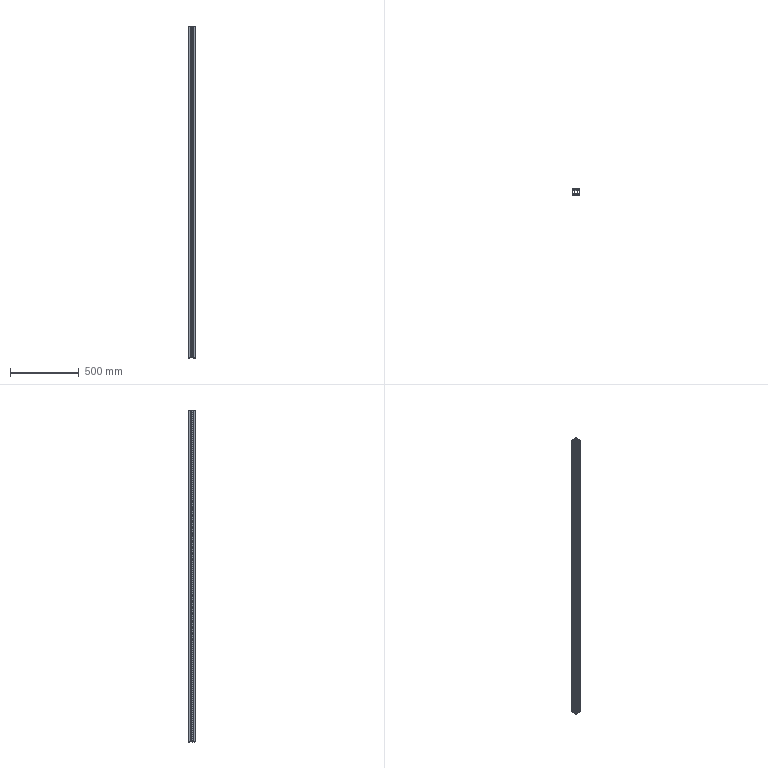Part | STEP file | 46A-00006CC11-2410mm | 1 solid | 142 faces | box 50 x 50 x 2410 mm | volume 1415857 mm3 | cylinder 84 | plane 58 | commonest cylinder face diameters 1 x24 4 x24 1.5 x16 3.7 x8 6.7 x8 2 x4